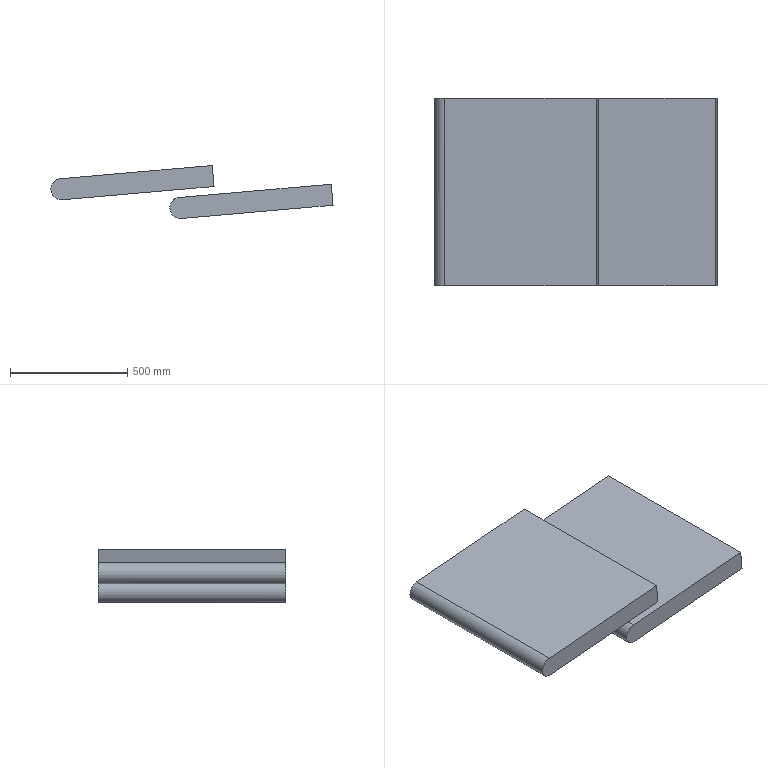Part | CATIA | 2 solids | 14 faces | box 1204 x 800 x 226.48 mm | volume 98689379 mm3 | plane 10 | cylinder 4 | commonest cylinder face diameters 90 x4
STEP:
#1=CARTESIAN_POINT('',(1712.527,-400.,186.651));
#2=VERTEX_POINT('',#1);
#3=CARTESIAN_POINT('',(1065.,-400.,130.));
#4=VERTEX_POINT('',#3);
#5=CARTESIAN_POINT('',(1388.763,-400.,158.326));
#6=DIRECTION('',(-0.9962,0.,-0.08716));
#7=VECTOR('',#6,1.);
#8=LINE('',#5,#7);
#9=EDGE_CURVE('',#2,#4,#8,.T.);
#10=ORIENTED_EDGE('',*,*,#9,.F.);
#11=CARTESIAN_POINT('',(1712.527,400.,186.651));
#12=VERTEX_POINT('',#11);
#13=CARTESIAN_POINT('',(1712.527,0.,186.651));
#14=DIRECTION('',(0.,1.,0.));
#15=VECTOR('',#14,1.);
#16=LINE('',#13,#15);
#17=EDGE_CURVE('',#2,#12,#16,.T.);
#18=ORIENTED_EDGE('',*,*,#17,.T.);
#19=CARTESIAN_POINT('',(1065.,400.,130.));
#20=VERTEX_POINT('',#19);
#21=CARTESIAN_POINT('',(1388.763,400.,158.326));
#22=DIRECTION('',(0.9962,0.,0.08716));
#23=VECTOR('',#22,1.);
#24=LINE('',#21,#23);
#25=EDGE_CURVE('',#20,#12,#24,.T.);
#26=ORIENTED_EDGE('',*,*,#25,.F.);
#27=CARTESIAN_POINT('',(1065.,0.,130.));
#28=DIRECTION('',(0.,-1.,0.));
#29=VECTOR('',#28,1.);
#30=LINE('',#27,#29);
#31=EDGE_CURVE('',#20,#4,#30,.T.);
#32=ORIENTED_EDGE('',*,*,#31,.T.);
#33=EDGE_LOOP('',(#10,#18,#26,#32));
#34=FACE_OUTER_BOUND('',#33,.T.);
#35=CARTESIAN_POINT('',(1065.,0.,130.));
#36=DIRECTION('',(-0.08716,0.,0.9962));
#37=DIRECTION('',(0.9962,0.,0.08716));
#38=AXIS2_PLACEMENT_3D('',#35,#36,#37);
#39=PLANE('',#38);
#40=ADVANCED_FACE('',(#34),#39,.T.);
#41=CARTESIAN_POINT('',(1072.844,-400.,40.342));
#42=VERTEX_POINT('',#41);
#43=CARTESIAN_POINT('',(1720.371,-400.,96.994));
#44=VERTEX_POINT('',#43);
#45=CARTESIAN_POINT('',(1396.607,-400.,68.668));
#46=DIRECTION('',(0.9962,0.,0.08716));
#47=VECTOR('',#46,1.);
#48=LINE('',#45,#47);
#49=EDGE_CURVE('',#42,#44,#48,.T.);
#50=ORIENTED_EDGE('',*,*,#49,.T.);
#51=CARTESIAN_POINT('',(1716.449,-400.,141.822));
#52=DIRECTION('',(-0.08716,0.,0.9962));
#53=VECTOR('',#52,1.);
#54=LINE('',#51,#53);
#55=EDGE_CURVE('',#44,#2,#54,.T.);
#56=ORIENTED_EDGE('',*,*,#55,.T.);
#57=ORIENTED_EDGE('',*,*,#9,.T.);
#58=CARTESIAN_POINT('',(1068.922,-400.,40.171));
#59=VERTEX_POINT('',#58);
#60=CARTESIAN_POINT('',(1068.922,-400.,40.171));
#61=CARTESIAN_POINT('',(1064.65,-400.,40.171));
#62=CARTESIAN_POINT('',(1060.378,-400.,40.678));
#63=CARTESIAN_POINT('',(1056.185,-400.,41.692));
#64=CARTESIAN_POINT('',(1048.122,-400.,44.696));
#65=CARTESIAN_POINT('',(1040.986,-400.,49.503));
#66=CARTESIAN_POINT('',(1037.721,-400.,52.321));
#67=CARTESIAN_POINT('',(1031.922,-400.,58.678));
#68=CARTESIAN_POINT('',(1027.772,-400.,66.215));
#69=CARTESIAN_POINT('',(1026.156,-400.,70.214));
#70=CARTESIAN_POINT('',(1023.904,-400.,78.518));
#71=CARTESIAN_POINT('',(1023.658,-400.,87.119));
#72=CARTESIAN_POINT('',(1024.048,-400.,91.414));
#73=CARTESIAN_POINT('',(1025.841,-400.,99.83));
#74=CARTESIAN_POINT('',(1029.553,-400.,107.592));
#75=CARTESIAN_POINT('',(1031.863,-400.,111.234));
#76=CARTESIAN_POINT('',(1037.304,-400.,117.9));
#77=CARTESIAN_POINT('',(1044.154,-400.,123.108));
#78=CARTESIAN_POINT('',(1047.873,-400.,125.291));
#79=CARTESIAN_POINT('',(1053.529,-400.,127.759));
#80=CARTESIAN_POINT('',(1059.486,-400.,129.23));
#81=CARTESIAN_POINT('',(1061.311,-400.,129.581));
#82=CARTESIAN_POINT('',(1063.151,-400.,129.838));
#83=CARTESIAN_POINT('',(1065.,-400.,130.));
#84=B_SPLINE_CURVE_WITH_KNOTS('',5,(#60,#61,#62,#63,#64,#65,#66,#67,#68,#69,#70,#71,#72,#73,#74,#75,#76,#77,#78,#79,#80,#81,#82,#83),.UNSPECIFIED.,.F.,.U.,(6,3,3,3,3,3,3,6),(0.,30.273,60.546,90.819,121.092,151.365,181.638,194.786),.UNSPECIFIED.);
#85=EDGE_CURVE('',#59,#4,#84,.T.);
#86=ORIENTED_EDGE('',*,*,#85,.F.);
#87=CARTESIAN_POINT('',(1072.844,-400.,40.342));
#88=CARTESIAN_POINT('',(1072.062,-400.,40.274));
#89=CARTESIAN_POINT('',(1071.278,-400.,40.223));
#90=CARTESIAN_POINT('',(1070.493,-400.,40.188));
#91=CARTESIAN_POINT('',(1069.707,-400.,40.171));
#92=CARTESIAN_POINT('',(1068.922,-400.,40.171));
#93=B_SPLINE_CURVE_WITH_KNOTS('',5,(#87,#88,#89,#90,#91,#92),.UNSPECIFIED.,.F.,.U.,(6,6),(0.,5.553),.UNSPECIFIED.);
#94=EDGE_CURVE('',#42,#59,#93,.T.);
#95=ORIENTED_EDGE('',*,*,#94,.F.);
#96=EDGE_LOOP('',(#50,#56,#57,#86,#95));
#97=FACE_OUTER_BOUND('',#96,.T.);
#98=CARTESIAN_POINT('',(1073.716,-400.,30.381));
#99=DIRECTION('',(0.,-1.,0.));
#100=DIRECTION('',(0.08716,0.,-0.9962));
#101=AXIS2_PLACEMENT_3D('',#98,#99,#100);
#102=PLANE('',#101);
#103=ADVANCED_FACE('',(#97),#102,.T.);
#104=CARTESIAN_POINT('',(1720.371,400.,96.994));
#105=VERTEX_POINT('',#104);
#106=CARTESIAN_POINT('',(1720.371,0.,96.994));
#107=DIRECTION('',(0.,-1.,0.));
#108=VECTOR('',#107,1.);
#109=LINE('',#106,#108);
#110=EDGE_CURVE('',#105,#44,#109,.T.);
#111=ORIENTED_EDGE('',*,*,#110,.F.);
#112=CARTESIAN_POINT('',(1716.449,400.,141.822));
#113=DIRECTION('',(0.08716,0.,-0.9962));
#114=VECTOR('',#113,1.);
#115=LINE('',#112,#114);
#116=EDGE_CURVE('',#12,#105,#115,.T.);
#117=ORIENTED_EDGE('',*,*,#116,.F.);
#118=ORIENTED_EDGE('',*,*,#17,.F.);
#119=ORIENTED_EDGE('',*,*,#55,.F.);
#120=EDGE_LOOP('',(#111,#117,#118,#119));
#121=FACE_OUTER_BOUND('',#120,.T.);
#122=CARTESIAN_POINT('',(1716.884,0.,136.841));
#123=DIRECTION('',(0.9962,0.,0.08716));
#124=DIRECTION('',(0.08716,0.,-0.9962));
#125=AXIS2_PLACEMENT_3D('',#122,#123,#124);
#126=PLANE('',#125);
#127=ADVANCED_FACE('',(#121),#126,.T.);
#128=ORIENTED_EDGE('',*,*,#25,.T.);
#129=ORIENTED_EDGE('',*,*,#116,.T.);
#130=CARTESIAN_POINT('',(1072.844,400.,40.342));
#131=VERTEX_POINT('',#130);
#132=CARTESIAN_POINT('',(1396.607,400.,68.668));
#133=DIRECTION('',(-0.9962,0.,-0.08716));
#134=VECTOR('',#133,1.);
#135=LINE('',#132,#134);
#136=EDGE_CURVE('',#105,#131,#135,.T.);
#137=ORIENTED_EDGE('',*,*,#136,.T.);
#138=CARTESIAN_POINT('',(1068.922,400.,40.171));
#139=VERTEX_POINT('',#138);
#140=CARTESIAN_POINT('',(1068.922,400.,40.171));
#141=CARTESIAN_POINT('',(1069.707,400.,40.171));
#142=CARTESIAN_POINT('',(1070.493,400.,40.188));
#143=CARTESIAN_POINT('',(1071.278,400.,40.223));
#144=CARTESIAN_POINT('',(1072.062,400.,40.274));
#145=CARTESIAN_POINT('',(1072.844,400.,40.342));
#146=B_SPLINE_CURVE_WITH_KNOTS('',5,(#140,#141,#142,#143,#144,#145),.UNSPECIFIED.,.F.,.U.,(6,6),(0.,5.553),.UNSPECIFIED.);
#147=EDGE_CURVE('',#139,#131,#146,.T.);
#148=ORIENTED_EDGE('',*,*,#147,.F.);
#149=CARTESIAN_POINT('',(1065.,400.,130.));
#150=CARTESIAN_POINT('',(1060.744,400.,129.628));
#151=CARTESIAN_POINT('',(1056.533,400.,128.75));
#152=CARTESIAN_POINT('',(1052.444,400.,127.375));
#153=CARTESIAN_POINT('',(1044.674,400.,123.68));
#154=CARTESIAN_POINT('',(1037.984,400.,118.269));
#155=CARTESIAN_POINT('',(1034.977,400.,115.177));
#156=CARTESIAN_POINT('',(1029.754,400.,108.339));
#157=CARTESIAN_POINT('',(1026.277,400.,100.469));
#158=CARTESIAN_POINT('',(1025.015,400.,96.344));
#159=CARTESIAN_POINT('',(1023.495,400.,87.875));
#160=CARTESIAN_POINT('',(1024.,400.,79.286));
#161=CARTESIAN_POINT('',(1024.763,400.,75.041));
#162=CARTESIAN_POINT('',(1027.282,400.,66.813));
#163=CARTESIAN_POINT('',(1031.657,400.,59.404));
#164=CARTESIAN_POINT('',(1034.276,400.,55.977));
#165=CARTESIAN_POINT('',(1040.277,400.,49.811));
#166=CARTESIAN_POINT('',(1047.554,400.,45.221));
#167=CARTESIAN_POINT('',(1051.45,400.,43.37));
#168=CARTESIAN_POINT('',(1057.299,400.,41.403));
#169=CARTESIAN_POINT('',(1063.362,400.,40.458));
#170=CARTESIAN_POINT('',(1065.211,400.,40.267));
#171=CARTESIAN_POINT('',(1067.066,400.,40.171));
#172=CARTESIAN_POINT('',(1068.922,400.,40.171));
#173=B_SPLINE_CURVE_WITH_KNOTS('',5,(#149,#150,#151,#152,#153,#154,#155,#156,#157,#158,#159,#160,#161,#162,#163,#164,#165,#166,#167,#168,#169,#170,#171,#172),.UNSPECIFIED.,.F.,.U.,(6,3,3,3,3,3,3,6),(0.,30.276,60.551,90.827,121.103,151.379,181.654,194.805),.UNSPECIFIED.);
#174=EDGE_CURVE('',#20,#139,#173,.T.);
#175=ORIENTED_EDGE('',*,*,#174,.F.);
#176=EDGE_LOOP('',(#128,#129,#137,#148,#175));
#177=FACE_OUTER_BOUND('',#176,.T.);
#178=CARTESIAN_POINT('',(1073.716,400.,30.381));
#179=DIRECTION('',(0.,1.,0.));
#180=DIRECTION('',(-0.08716,0.,0.9962));
#181=AXIS2_PLACEMENT_3D('',#178,#179,#180);
#182=PLANE('',#181);
#183=ADVANCED_FACE('',(#177),#182,.T.);
#184=CARTESIAN_POINT('',(1068.922,0.,40.171));
#185=DIRECTION('',(0.,1.,0.));
#186=VECTOR('',#185,1.);
#187=LINE('',#184,#186);
#188=EDGE_CURVE('',#59,#139,#187,.T.);
#189=ORIENTED_EDGE('',*,*,#188,.F.);
#190=ORIENTED_EDGE('',*,*,#85,.T.);
#191=ORIENTED_EDGE('',*,*,#31,.F.);
#192=ORIENTED_EDGE('',*,*,#174,.T.);
#193=EDGE_LOOP('',(#189,#190,#191,#192));
#194=FACE_OUTER_BOUND('',#193,.T.);
#195=CARTESIAN_POINT('',(1068.922,0.,85.171));
#196=DIRECTION('',(0.,1.,0.));
#197=DIRECTION('',(0.,0.,-1.));
#198=AXIS2_PLACEMENT_3D('',#195,#196,#197);
#199=CYLINDRICAL_SURFACE('',#198,45.);
#200=ADVANCED_FACE('',(#194),#199,.T.);
#201=ORIENTED_EDGE('',*,*,#136,.F.);
#202=ORIENTED_EDGE('',*,*,#110,.T.);
#203=ORIENTED_EDGE('',*,*,#49,.F.);
#204=CARTESIAN_POINT('',(1072.844,0.,40.342));
#205=DIRECTION('',(0.,1.,0.));
#206=VECTOR('',#205,1.);
#207=LINE('',#204,#206);
#208=EDGE_CURVE('',#42,#131,#207,.T.);
#209=ORIENTED_EDGE('',*,*,#208,.T.);
#210=EDGE_LOOP('',(#201,#202,#203,#209));
#211=FACE_OUTER_BOUND('',#210,.T.);
#212=CARTESIAN_POINT('',(1072.844,0.,40.342));
#213=DIRECTION('',(0.08716,0.,-0.9962));
#214=DIRECTION('',(-0.9962,0.,-0.08716));
#215=AXIS2_PLACEMENT_3D('',#212,#213,#214);
#216=PLANE('',#215);
#217=ADVANCED_FACE('',(#211),#216,.T.);
#218=ORIENTED_EDGE('',*,*,#188,.T.);
#219=ORIENTED_EDGE('',*,*,#147,.T.);
#220=ORIENTED_EDGE('',*,*,#208,.F.);
#221=ORIENTED_EDGE('',*,*,#94,.T.);
#222=EDGE_LOOP('',(#218,#219,#220,#221));
#223=FACE_OUTER_BOUND('',#222,.T.);
#224=CARTESIAN_POINT('',(1068.922,0.,85.171));
#225=DIRECTION('',(0.,1.,0.));
#226=DIRECTION('',(0.,0.,1.));
#227=AXIS2_PLACEMENT_3D('',#224,#225,#226);
#228=CYLINDRICAL_SURFACE('',#227,45.);
#229=ADVANCED_FACE('',(#223),#228,.T.);
#230=CLOSED_SHELL('',(#40,#103,#127,#183,#200,#217,#229));
#231=MANIFOLD_SOLID_BREP('',#230);
#232=CARTESIAN_POINT('',(1204.527,-400.,266.651));
#233=VERTEX_POINT('',#232);
#234=CARTESIAN_POINT('',(557.,-400.,210.));
#235=VERTEX_POINT('',#234);
#236=CARTESIAN_POINT('',(880.763,-400.,238.326));
#237=DIRECTION('',(-0.9962,0.,-0.08716));
#238=VECTOR('',#237,1.);
#239=LINE('',#236,#238);
#240=EDGE_CURVE('',#233,#235,#239,.T.);
#241=ORIENTED_EDGE('',*,*,#240,.F.);
#242=CARTESIAN_POINT('',(1204.527,400.,266.651));
#243=VERTEX_POINT('',#242);
#244=CARTESIAN_POINT('',(1204.527,0.,266.651));
#245=DIRECTION('',(0.,1.,0.));
#246=VECTOR('',#245,1.);
#247=LINE('',#244,#246);
#248=EDGE_CURVE('',#233,#243,#247,.T.);
#249=ORIENTED_EDGE('',*,*,#248,.T.);
#250=CARTESIAN_POINT('',(557.,400.,210.));
#251=VERTEX_POINT('',#250);
#252=CARTESIAN_POINT('',(880.763,400.,238.326));
#253=DIRECTION('',(0.9962,0.,0.08716));
#254=VECTOR('',#253,1.);
#255=LINE('',#252,#254);
#256=EDGE_CURVE('',#251,#243,#255,.T.);
#257=ORIENTED_EDGE('',*,*,#256,.F.);
#258=CARTESIAN_POINT('',(557.,0.,210.));
#259=DIRECTION('',(0.,-1.,0.));
#260=VECTOR('',#259,1.);
#261=LINE('',#258,#260);
#262=EDGE_CURVE('',#251,#235,#261,.T.);
#263=ORIENTED_EDGE('',*,*,#262,.T.);
#264=EDGE_LOOP('',(#241,#249,#257,#263));
#265=FACE_OUTER_BOUND('',#264,.T.);
#266=CARTESIAN_POINT('',(557.,0.,210.));
#267=DIRECTION('',(-0.08716,0.,0.9962));
#268=DIRECTION('',(0.9962,0.,0.08716));
#269=AXIS2_PLACEMENT_3D('',#266,#267,#268);
#270=PLANE('',#269);
#271=ADVANCED_FACE('',(#265),#270,.T.);
#272=CARTESIAN_POINT('',(564.844,-400.,120.342));
#273=VERTEX_POINT('',#272);
#274=CARTESIAN_POINT('',(1212.371,-400.,176.994));
#275=VERTEX_POINT('',#274);
#276=CARTESIAN_POINT('',(888.607,-400.,148.668));
#277=DIRECTION('',(0.9962,0.,0.08716));
#278=VECTOR('',#277,1.);
#279=LINE('',#276,#278);
#280=EDGE_CURVE('',#273,#275,#279,.T.);
#281=ORIENTED_EDGE('',*,*,#280,.T.);
#282=CARTESIAN_POINT('',(1208.449,-400.,221.822));
#283=DIRECTION('',(-0.08716,0.,0.9962));
#284=VECTOR('',#283,1.);
#285=LINE('',#282,#284);
#286=EDGE_CURVE('',#275,#233,#285,.T.);
#287=ORIENTED_EDGE('',*,*,#286,.T.);
#288=ORIENTED_EDGE('',*,*,#240,.T.);
#289=CARTESIAN_POINT('',(560.922,-400.,120.171));
#290=VERTEX_POINT('',#289);
#291=CARTESIAN_POINT('',(560.922,-400.,120.171));
#292=CARTESIAN_POINT('',(556.65,-400.,120.171));
#293=CARTESIAN_POINT('',(552.378,-400.,120.678));
#294=CARTESIAN_POINT('',(548.185,-400.,121.692));
#295=CARTESIAN_POINT('',(540.122,-400.,124.696));
#296=CARTESIAN_POINT('',(532.986,-400.,129.503));
#297=CARTESIAN_POINT('',(529.721,-400.,132.321));
#298=CARTESIAN_POINT('',(523.922,-400.,138.678));
#299=CARTESIAN_POINT('',(519.772,-400.,146.215));
#300=CARTESIAN_POINT('',(518.156,-400.,150.214));
#301=CARTESIAN_POINT('',(515.904,-400.,158.518));
#302=CARTESIAN_POINT('',(515.658,-400.,167.119));
#303=CARTESIAN_POINT('',(516.048,-400.,171.414));
#304=CARTESIAN_POINT('',(517.841,-400.,179.83));
#305=CARTESIAN_POINT('',(521.553,-400.,187.592));
#306=CARTESIAN_POINT('',(523.863,-400.,191.234));
#307=CARTESIAN_POINT('',(529.304,-400.,197.9));
#308=CARTESIAN_POINT('',(536.154,-400.,203.108));
#309=CARTESIAN_POINT('',(539.873,-400.,205.291));
#310=CARTESIAN_POINT('',(545.529,-400.,207.759));
#311=CARTESIAN_POINT('',(551.486,-400.,209.23));
#312=CARTESIAN_POINT('',(553.311,-400.,209.581));
#313=CARTESIAN_POINT('',(555.151,-400.,209.838));
#314=CARTESIAN_POINT('',(557.,-400.,210.));
#315=B_SPLINE_CURVE_WITH_KNOTS('',5,(#291,#292,#293,#294,#295,#296,#297,#298,#299,#300,#301,#302,#303,#304,#305,#306,#307,#308,#309,#310,#311,#312,#313,#314),.UNSPECIFIED.,.F.,.U.,(6,3,3,3,3,3,3,6),(0.,30.273,60.546,90.819,121.092,151.365,181.638,194.786),.UNSPECIFIED.);
#316=EDGE_CURVE('',#290,#235,#315,.T.);
#317=ORIENTED_EDGE('',*,*,#316,.F.);
#318=CARTESIAN_POINT('',(564.844,-400.,120.342));
#319=CARTESIAN_POINT('',(564.062,-400.,120.274));
#320=CARTESIAN_POINT('',(563.278,-400.,120.223));
#321=CARTESIAN_POINT('',(562.493,-400.,120.188));
#322=CARTESIAN_POINT('',(561.707,-400.,120.171));
#323=CARTESIAN_POINT('',(560.922,-400.,120.171));
#324=B_SPLINE_CURVE_WITH_KNOTS('',5,(#318,#319,#320,#321,#322,#323),.UNSPECIFIED.,.F.,.U.,(6,6),(0.,5.553),.UNSPECIFIED.);
#325=EDGE_CURVE('',#273,#290,#324,.T.);
#326=ORIENTED_EDGE('',*,*,#325,.F.);
#327=EDGE_LOOP('',(#281,#287,#288,#317,#326));
#328=FACE_OUTER_BOUND('',#327,.T.);
#329=CARTESIAN_POINT('',(565.716,-400.,110.381));
#330=DIRECTION('',(0.,-1.,0.));
#331=DIRECTION('',(0.08716,0.,-0.9962));
#332=AXIS2_PLACEMENT_3D('',#329,#330,#331);
#333=PLANE('',#332);
#334=ADVANCED_FACE('',(#328),#333,.T.);
#335=CARTESIAN_POINT('',(1212.371,400.,176.994));
#336=VERTEX_POINT('',#335);
#337=CARTESIAN_POINT('',(1212.371,0.,176.994));
#338=DIRECTION('',(0.,-1.,0.));
#339=VECTOR('',#338,1.);
#340=LINE('',#337,#339);
#341=EDGE_CURVE('',#336,#275,#340,.T.);
#342=ORIENTED_EDGE('',*,*,#341,.F.);
#343=CARTESIAN_POINT('',(1208.449,400.,221.822));
#344=DIRECTION('',(0.08716,0.,-0.9962));
#345=VECTOR('',#344,1.);
#346=LINE('',#343,#345);
#347=EDGE_CURVE('',#243,#336,#346,.T.);
#348=ORIENTED_EDGE('',*,*,#347,.F.);
#349=ORIENTED_EDGE('',*,*,#248,.F.);
#350=ORIENTED_EDGE('',*,*,#286,.F.);
#351=EDGE_LOOP('',(#342,#348,#349,#350));
#352=FACE_OUTER_BOUND('',#351,.T.);
#353=CARTESIAN_POINT('',(1208.884,0.,216.841));
#354=DIRECTION('',(0.9962,0.,0.08716));
#355=DIRECTION('',(0.08716,0.,-0.9962));
#356=AXIS2_PLACEMENT_3D('',#353,#354,#355);
#357=PLANE('',#356);
#358=ADVANCED_FACE('',(#352),#357,.T.);
#359=ORIENTED_EDGE('',*,*,#256,.T.);
#360=ORIENTED_EDGE('',*,*,#347,.T.);
#361=CARTESIAN_POINT('',(564.844,400.,120.342));
#362=VERTEX_POINT('',#361);
#363=CARTESIAN_POINT('',(888.607,400.,148.668));
#364=DIRECTION('',(-0.9962,0.,-0.08716));
#365=VECTOR('',#364,1.);
#366=LINE('',#363,#365);
#367=EDGE_CURVE('',#336,#362,#366,.T.);
#368=ORIENTED_EDGE('',*,*,#367,.T.);
#369=CARTESIAN_POINT('',(560.922,400.,120.171));
#370=VERTEX_POINT('',#369);
#371=CARTESIAN_POINT('',(560.922,400.,120.171));
#372=CARTESIAN_POINT('',(561.707,400.,120.171));
#373=CARTESIAN_POINT('',(562.493,400.,120.188));
#374=CARTESIAN_POINT('',(563.278,400.,120.223));
#375=CARTESIAN_POINT('',(564.062,400.,120.274));
#376=CARTESIAN_POINT('',(564.844,400.,120.342));
#377=B_SPLINE_CURVE_WITH_KNOTS('',5,(#371,#372,#373,#374,#375,#376),.UNSPECIFIED.,.F.,.U.,(6,6),(0.,5.553),.UNSPECIFIED.);
#378=EDGE_CURVE('',#370,#362,#377,.T.);
#379=ORIENTED_EDGE('',*,*,#378,.F.);
#380=CARTESIAN_POINT('',(557.,400.,210.));
#381=CARTESIAN_POINT('',(552.744,400.,209.628));
#382=CARTESIAN_POINT('',(548.533,400.,208.75));
#383=CARTESIAN_POINT('',(544.444,400.,207.375));
#384=CARTESIAN_POINT('',(536.674,400.,203.68));
#385=CARTESIAN_POINT('',(529.984,400.,198.269));
#386=CARTESIAN_POINT('',(526.977,400.,195.177));
#387=CARTESIAN_POINT('',(521.754,400.,188.339));
#388=CARTESIAN_POINT('',(518.277,400.,180.469));
#389=CARTESIAN_POINT('',(517.015,400.,176.344));
#390=CARTESIAN_POINT('',(515.495,400.,167.875));
#391=CARTESIAN_POINT('',(516.,400.,159.286));
#392=CARTESIAN_POINT('',(516.763,400.,155.041));
#393=CARTESIAN_POINT('',(519.282,400.,146.813));
#394=CARTESIAN_POINT('',(523.657,400.,139.404));
#395=CARTESIAN_POINT('',(526.276,400.,135.977));
#396=CARTESIAN_POINT('',(532.277,400.,129.811));
#397=CARTESIAN_POINT('',(539.554,400.,125.221));
#398=CARTESIAN_POINT('',(543.45,400.,123.37));
#399=CARTESIAN_POINT('',(549.299,400.,121.403));
#400=CARTESIAN_POINT('',(555.362,400.,120.458));
#401=CARTESIAN_POINT('',(557.211,400.,120.267));
#402=CARTESIAN_POINT('',(559.066,400.,120.171));
#403=CARTESIAN_POINT('',(560.922,400.,120.171));
#404=B_SPLINE_CURVE_WITH_KNOTS('',5,(#380,#381,#382,#383,#384,#385,#386,#387,#388,#389,#390,#391,#392,#393,#394,#395,#396,#397,#398,#399,#400,#401,#402,#403),.UNSPECIFIED.,.F.,.U.,(6,3,3,3,3,3,3,6),(0.,30.276,60.551,90.827,121.103,151.379,181.654,194.805),.UNSPECIFIED.);
#405=EDGE_CURVE('',#251,#370,#404,.T.);
#406=ORIENTED_EDGE('',*,*,#405,.F.);
#407=EDGE_LOOP('',(#359,#360,#368,#379,#406));
#408=FACE_OUTER_BOUND('',#407,.T.);
#409=CARTESIAN_POINT('',(565.716,400.,110.381));
#410=DIRECTION('',(0.,1.,0.));
#411=DIRECTION('',(-0.08716,0.,0.9962));
#412=AXIS2_PLACEMENT_3D('',#409,#410,#411);
#413=PLANE('',#412);
#414=ADVANCED_FACE('',(#408),#413,.T.);
#415=CARTESIAN_POINT('',(560.922,0.,120.171));
#416=DIRECTION('',(0.,1.,0.));
#417=VECTOR('',#416,1.);
#418=LINE('',#415,#417);
#419=EDGE_CURVE('',#290,#370,#418,.T.);
#420=ORIENTED_EDGE('',*,*,#419,.F.);
#421=ORIENTED_EDGE('',*,*,#316,.T.);
#422=ORIENTED_EDGE('',*,*,#262,.F.);
#423=ORIENTED_EDGE('',*,*,#405,.T.);
#424=EDGE_LOOP('',(#420,#421,#422,#423));
#425=FACE_OUTER_BOUND('',#424,.T.);
#426=CARTESIAN_POINT('',(560.922,0.,165.171));
#427=DIRECTION('',(0.,1.,0.));
#428=DIRECTION('',(0.,0.,-1.));
#429=AXIS2_PLACEMENT_3D('',#426,#427,#428);
#430=CYLINDRICAL_SURFACE('',#429,45.);
#431=ADVANCED_FACE('',(#425),#430,.T.);
#432=ORIENTED_EDGE('',*,*,#367,.F.);
#433=ORIENTED_EDGE('',*,*,#341,.T.);
#434=ORIENTED_EDGE('',*,*,#280,.F.);
#435=CARTESIAN_POINT('',(564.844,0.,120.342));
#436=DIRECTION('',(0.,1.,0.));
#437=VECTOR('',#436,1.);
#438=LINE('',#435,#437);
#439=EDGE_CURVE('',#273,#362,#438,.T.);
#440=ORIENTED_EDGE('',*,*,#439,.T.);
#441=EDGE_LOOP('',(#432,#433,#434,#440));
#442=FACE_OUTER_BOUND('',#441,.T.);
#443=CARTESIAN_POINT('',(564.844,0.,120.342));
#444=DIRECTION('',(0.08716,0.,-0.9962));
#445=DIRECTION('',(-0.9962,0.,-0.08716));
#446=AXIS2_PLACEMENT_3D('',#443,#444,#445);
#447=PLANE('',#446);
#448=ADVANCED_FACE('',(#442),#447,.T.);
#449=ORIENTED_EDGE('',*,*,#419,.T.);
#450=ORIENTED_EDGE('',*,*,#378,.T.);
#451=ORIENTED_EDGE('',*,*,#439,.F.);
#452=ORIENTED_EDGE('',*,*,#325,.T.);
#453=EDGE_LOOP('',(#449,#450,#451,#452));
#454=FACE_OUTER_BOUND('',#453,.T.);
#455=CARTESIAN_POINT('',(560.922,0.,165.171));
#456=DIRECTION('',(0.,1.,0.));
#457=DIRECTION('',(0.,0.,1.));
#458=AXIS2_PLACEMENT_3D('',#455,#456,#457);
#459=CYLINDRICAL_SURFACE('',#458,45.);
#460=ADVANCED_FACE('',(#454),#459,.T.);
#461=CLOSED_SHELL('',(#271,#334,#358,#414,#431,#448,#460));
#462=MANIFOLD_SOLID_BREP('',#461);
#463=(LENGTH_UNIT()NAMED_UNIT(*)SI_UNIT(.MILLI.,.METRE.));
#464=UNCERTAINTY_MEASURE_WITH_UNIT(LENGTH_MEASURE(0.005),#463,'','');
#465=(NAMED_UNIT(*)PLANE_ANGLE_UNIT()SI_UNIT($,.RADIAN.));
#466=(NAMED_UNIT(*)SI_UNIT($,.STERADIAN.)SOLID_ANGLE_UNIT());
#467=(GEOMETRIC_REPRESENTATION_CONTEXT(3)GLOBAL_UNCERTAINTY_ASSIGNED_CONTEXT((#464))GLOBAL_UNIT_ASSIGNED_CONTEXT((#463,#465,#466))REPRESENTATION_CONTEXT('',''));
#468=ADVANCED_BREP_SHAPE_REPRESENTATION('',(#231,#462),#467);